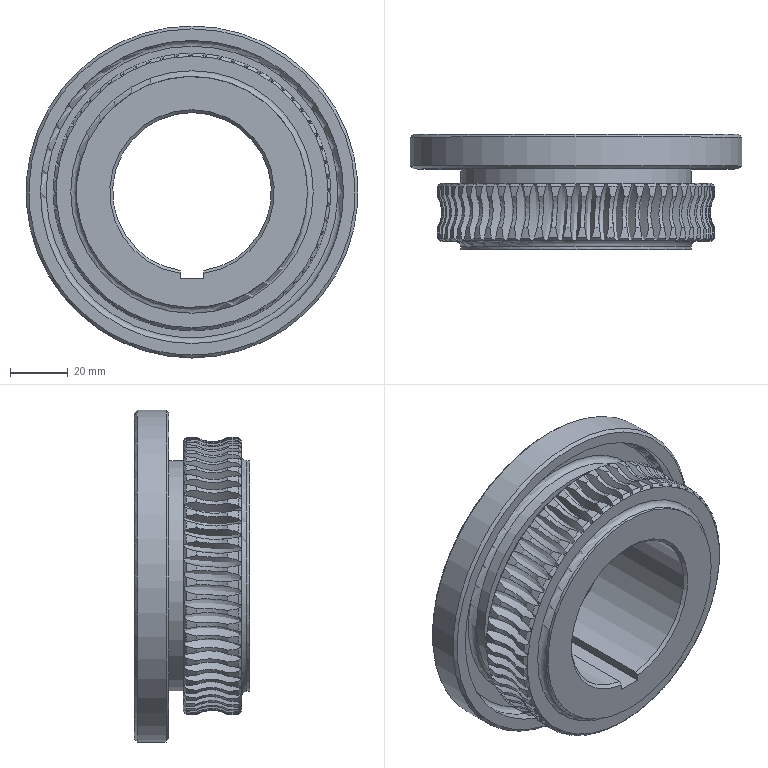Part | NX | features DATUM_CSYS 10, SKETCH 9, EXTRUDE 6, CHAMFER 3, BLEND 2, ASSOCIATIVE_INTERSECTION 1, DATUM_PLANE 1, INTERSECT 1, Pattern Face Feature 1, SKIN 1, SUBTRACT 1, SWP104 1 | 1 solid | 265 faces | box 115 x 40 x 115 mm | volume 186208 mm3 | cylinder 126 | torus 63 | spline 60 | plane 10 | cone 6 | commonest cylinder face diameters 96 x120 80 x2 55 x1 86 x1 105 x1 115 x1